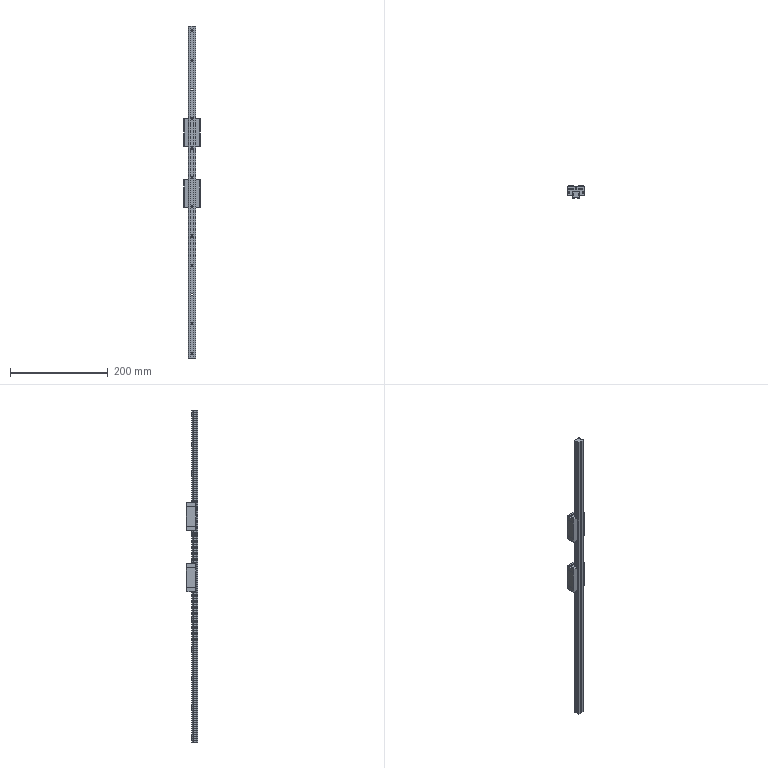Part | SolidWorks | 3 solids | 906 faces | box 34 x 24 x 680 mm | volume 167801 mm3 | plane 574 | cylinder 196 | spline 136 | commonest cylinder face diameters 1.6 x32 2.1 x24 4 x24 4.5 x24 8 x24 0.6 x19